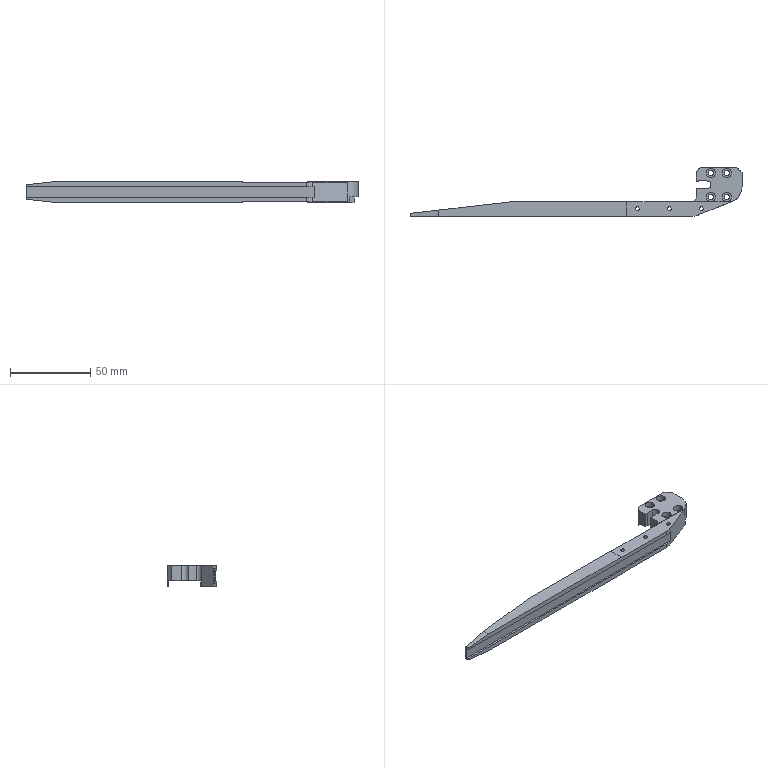NC program | NX | posted by the shop | part box 207.5 x 30.8 x 13 mm
Lines 1 to 85 of 6162:
%
O0001
(Machine time: 207.83 MIN)
(===Total Tool:9===)
(T1=D80R0.8 fly cutter D=80.  R=0.8  D-  H01 Z=0.    )
(T2=D6 chamfer cutter   D=6.   R=0.   D-  H02 Z=-4.9  )
(T12=ZT2.5  D=2.5  DR_a=118 D-  H12 Z=-18.45)
(T13=ZT3.4  D=3.4  DR_a=118 D-  H13 Z=-12.62)
(T9=D10     D=10.  R=0.   D-  H09 Z=-13.1 )
(T7=D6-J    D=6.   R=0.   D-  H07 Z=-13.  )
(T17=D3-J   D=3.   R=0.   D-  H17 Z=-12.95)
(T18=R2     D=4.   R=2.   D-  H18 Z=-2.08 )
(T20=M3X0.5 D=2.5  DR_a=180 D-  H20 Z=-15.7 )
G80 G90 G17 G49 G40
G91 G28 Z0
M01
N1 T01 M06
(D80R0.8 fly cutter  D=80. R=0.8 H=01 ce=0.00 di=0.00)
G00 G90 G54 X-148.75 Y0.0 M03 S4000
G43 H01 Z20.
M08
Z2.
G01 Z0.0 F1000.
X-143.75
X143.75
X148.75
Z2.
G00 Z20.
G91 G28 Z0.0
M05
M09
G91 G28 Z0.0
M01
N2 T02 M06
(D6 chamfer cutter  D=6. R=0. H=02 ce=0.00 di=0.00)
G00 G90 G54 X-38.25 Y-10.4 M03 S8000
G43 H02 Z20.
M08
G98 G81 X-38.25 Y-10.4 Z-.8 R1. F500.
X-58.25
X-78.25
X-84.25 Y-3.1
X-94.25
Y11.9
X-84.25
G80
G00 Z20.
G91 G28 Z0.0
M05
M09
G91 G28 Z0.0
M01
N3 T12 M06
(ZT2.5 D=2.5 DR_a=118 H=12)
G00 G90 G54 X-78.25 Y-10.4 M03 S3000
G43 H12 Z20.
M08
G98 G83 X-78.25 Y-10.4 Z-18.451 R1. F300. Q2.
X-58.25
X-38.25
G80
G00 Z20.
G91 G28 Z0.0
M05
M09
G91 G28 Z0.0
M01
N4 T13 M06
(ZT3.4 D=3.4 DR_a=118 H=13)
G00 G90 G54 X-94.25 Y-3.1 M03 S3000
G43 H13 Z20.
M08
G98 G83 X-94.25 Y-3.1 Z-12.621 R1. F120. Q3.
X-84.25
Y11.9
X-94.25
G80
G00 Z20.
G91 G28 Z0.0
M05
M09
G91 G28 Z0.0
M01